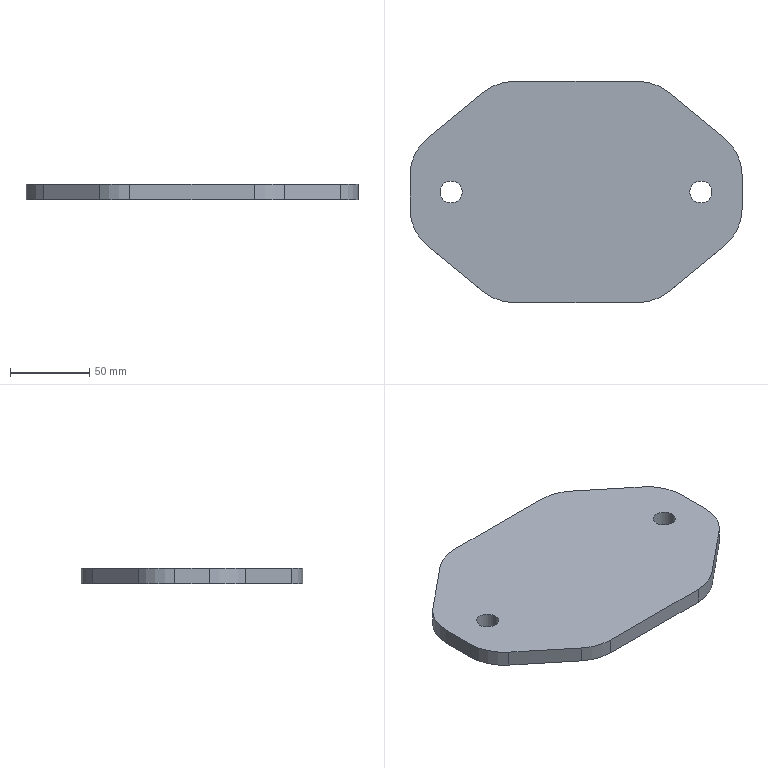Part | STEP file | VD-SYL0380DJ1006_1_1_2-3_VD-SYL | 1 solid | 22 faces | box 210 x 140 x 10 mm | volume 239785 mm3 | cylinder 12 | plane 10 | commonest cylinder face diameters 60 x8 14 x4
STEP:
#1=CARTESIAN_POINT('',(86.,0.,0.));
#2=VERTEX_POINT('',#1);
#3=CARTESIAN_POINT('',(72.,0.,0.));
#4=VERTEX_POINT('',#3);
#5=CARTESIAN_POINT('',(79.,0.,0.));
#6=DIRECTION('',(0.,0.,1.));
#7=DIRECTION('',(1.,0.,0.));
#8=AXIS2_PLACEMENT_3D('',#5,#6,#7);
#9=CIRCLE('',#8,7.);
#10=EDGE_CURVE('',#2,#4,#9,.T.);
#11=ORIENTED_EDGE('',*,*,#10,.F.);
#12=CARTESIAN_POINT('',(86.,0.,10.));
#13=VERTEX_POINT('',#12);
#14=CARTESIAN_POINT('',(86.,0.,10.));
#15=DIRECTION('',(0.,0.,-1.));
#16=VECTOR('',#15,1000.);
#17=LINE('',#14,#16);
#18=EDGE_CURVE('',#13,#2,#17,.T.);
#19=ORIENTED_EDGE('',*,*,#18,.F.);
#20=CARTESIAN_POINT('',(72.,0.,10.));
#21=VERTEX_POINT('',#20);
#22=CARTESIAN_POINT('',(79.,0.,10.));
#23=DIRECTION('',(0.,0.,-1.));
#24=DIRECTION('',(-1.,0.,0.));
#25=AXIS2_PLACEMENT_3D('',#22,#23,#24);
#26=CIRCLE('',#25,7.);
#27=EDGE_CURVE('',#21,#13,#26,.T.);
#28=ORIENTED_EDGE('',*,*,#27,.F.);
#29=CARTESIAN_POINT('',(72.,0.,10.));
#30=DIRECTION('',(0.,0.,-1.));
#31=VECTOR('',#30,1000.);
#32=LINE('',#29,#31);
#33=EDGE_CURVE('',#21,#4,#32,.T.);
#34=ORIENTED_EDGE('',*,*,#33,.T.);
#35=EDGE_LOOP('',(#11,#19,#28,#34));
#36=FACE_OUTER_BOUND('',#35,.T.);
#37=CARTESIAN_POINT('',(79.,0.,5.));
#38=DIRECTION('',(0.,0.,1.));
#39=DIRECTION('',(1.,0.,0.));
#40=AXIS2_PLACEMENT_3D('',#37,#38,#39);
#41=CYLINDRICAL_SURFACE('',#40,7.);
#42=ADVANCED_FACE('',(#36),#41,.F.);
#43=ORIENTED_EDGE('',*,*,#33,.F.);
#44=CARTESIAN_POINT('',(79.,0.,10.));
#45=DIRECTION('',(0.,0.,-1.));
#46=DIRECTION('',(1.,0.,0.));
#47=AXIS2_PLACEMENT_3D('',#44,#45,#46);
#48=CIRCLE('',#47,7.);
#49=EDGE_CURVE('',#13,#21,#48,.T.);
#50=ORIENTED_EDGE('',*,*,#49,.F.);
#51=ORIENTED_EDGE('',*,*,#18,.T.);
#52=CARTESIAN_POINT('',(79.,0.,0.));
#53=DIRECTION('',(0.,0.,1.));
#54=DIRECTION('',(-1.,0.,0.));
#55=AXIS2_PLACEMENT_3D('',#52,#53,#54);
#56=CIRCLE('',#55,7.);
#57=EDGE_CURVE('',#4,#2,#56,.T.);
#58=ORIENTED_EDGE('',*,*,#57,.F.);
#59=EDGE_LOOP('',(#43,#50,#51,#58));
#60=FACE_OUTER_BOUND('',#59,.T.);
#61=CARTESIAN_POINT('',(79.,0.,5.));
#62=DIRECTION('',(0.,0.,1.));
#63=DIRECTION('',(1.,0.,0.));
#64=AXIS2_PLACEMENT_3D('',#61,#62,#63);
#65=CYLINDRICAL_SURFACE('',#64,7.);
#66=ADVANCED_FACE('',(#60),#65,.F.);
#67=CARTESIAN_POINT('',(-72.,0.,0.));
#68=VERTEX_POINT('',#67);
#69=CARTESIAN_POINT('',(-86.,0.,0.));
#70=VERTEX_POINT('',#69);
#71=CARTESIAN_POINT('',(-79.,0.,0.));
#72=DIRECTION('',(0.,0.,1.));
#73=DIRECTION('',(1.,0.,0.));
#74=AXIS2_PLACEMENT_3D('',#71,#72,#73);
#75=CIRCLE('',#74,7.);
#76=EDGE_CURVE('',#68,#70,#75,.T.);
#77=ORIENTED_EDGE('',*,*,#76,.F.);
#78=CARTESIAN_POINT('',(-72.,0.,10.));
#79=VERTEX_POINT('',#78);
#80=CARTESIAN_POINT('',(-72.,0.,10.));
#81=DIRECTION('',(0.,0.,-1.));
#82=VECTOR('',#81,1000.);
#83=LINE('',#80,#82);
#84=EDGE_CURVE('',#79,#68,#83,.T.);
#85=ORIENTED_EDGE('',*,*,#84,.F.);
#86=CARTESIAN_POINT('',(-86.,0.,10.));
#87=VERTEX_POINT('',#86);
#88=CARTESIAN_POINT('',(-79.,0.,10.));
#89=DIRECTION('',(0.,0.,-1.));
#90=DIRECTION('',(-1.,0.,0.));
#91=AXIS2_PLACEMENT_3D('',#88,#89,#90);
#92=CIRCLE('',#91,7.);
#93=EDGE_CURVE('',#87,#79,#92,.T.);
#94=ORIENTED_EDGE('',*,*,#93,.F.);
#95=CARTESIAN_POINT('',(-86.,0.,10.));
#96=DIRECTION('',(0.,0.,-1.));
#97=VECTOR('',#96,1000.);
#98=LINE('',#95,#97);
#99=EDGE_CURVE('',#87,#70,#98,.T.);
#100=ORIENTED_EDGE('',*,*,#99,.T.);
#101=EDGE_LOOP('',(#77,#85,#94,#100));
#102=FACE_OUTER_BOUND('',#101,.T.);
#103=CARTESIAN_POINT('',(-79.,0.,5.));
#104=DIRECTION('',(0.,0.,1.));
#105=DIRECTION('',(1.,0.,0.));
#106=AXIS2_PLACEMENT_3D('',#103,#104,#105);
#107=CYLINDRICAL_SURFACE('',#106,7.);
#108=ADVANCED_FACE('',(#102),#107,.F.);
#109=ORIENTED_EDGE('',*,*,#99,.F.);
#110=CARTESIAN_POINT('',(-79.,0.,10.));
#111=DIRECTION('',(0.,0.,-1.));
#112=DIRECTION('',(1.,0.,0.));
#113=AXIS2_PLACEMENT_3D('',#110,#111,#112);
#114=CIRCLE('',#113,7.);
#115=EDGE_CURVE('',#79,#87,#114,.T.);
#116=ORIENTED_EDGE('',*,*,#115,.F.);
#117=ORIENTED_EDGE('',*,*,#84,.T.);
#118=CARTESIAN_POINT('',(-79.,0.,0.));
#119=DIRECTION('',(0.,0.,1.));
#120=DIRECTION('',(-1.,0.,0.));
#121=AXIS2_PLACEMENT_3D('',#118,#119,#120);
#122=CIRCLE('',#121,7.);
#123=EDGE_CURVE('',#70,#68,#122,.T.);
#124=ORIENTED_EDGE('',*,*,#123,.F.);
#125=EDGE_LOOP('',(#109,#116,#117,#124));
#126=FACE_OUTER_BOUND('',#125,.T.);
#127=CARTESIAN_POINT('',(-79.,0.,5.));
#128=DIRECTION('',(0.,0.,1.));
#129=DIRECTION('',(1.,0.,0.));
#130=AXIS2_PLACEMENT_3D('',#127,#128,#129);
#131=CYLINDRICAL_SURFACE('',#130,7.);
#132=ADVANCED_FACE('',(#126),#131,.F.);
#133=CARTESIAN_POINT('',(105.,-10.784,0.));
#134=VERTEX_POINT('',#133);
#135=CARTESIAN_POINT('',(93.997,-34.002,0.));
#136=VERTEX_POINT('',#135);
#137=CARTESIAN_POINT('',(75.,-10.784,0.));
#138=DIRECTION('',(0.,0.,-1.));
#139=DIRECTION('',(1.,0.,0.));
#140=AXIS2_PLACEMENT_3D('',#137,#138,#139);
#141=CIRCLE('',#140,30.);
#142=EDGE_CURVE('',#134,#136,#141,.T.);
#143=ORIENTED_EDGE('',*,*,#142,.F.);
#144=CARTESIAN_POINT('',(105.,-10.784,10.));
#145=VERTEX_POINT('',#144);
#146=CARTESIAN_POINT('',(105.,-10.784,0.));
#147=DIRECTION('',(0.,0.,1.));
#148=VECTOR('',#147,1000.);
#149=LINE('',#146,#148);
#150=EDGE_CURVE('',#134,#145,#149,.T.);
#151=ORIENTED_EDGE('',*,*,#150,.T.);
#152=CARTESIAN_POINT('',(93.997,-34.002,10.));
#153=VERTEX_POINT('',#152);
#154=CARTESIAN_POINT('',(75.,-10.784,10.));
#155=DIRECTION('',(0.,0.,1.));
#156=DIRECTION('',(0.6332,-0.774,0.));
#157=AXIS2_PLACEMENT_3D('',#154,#155,#156);
#158=CIRCLE('',#157,30.);
#159=EDGE_CURVE('',#153,#145,#158,.T.);
#160=ORIENTED_EDGE('',*,*,#159,.F.);
#161=CARTESIAN_POINT('',(93.997,-34.002,10.));
#162=DIRECTION('',(0.,0.,-1.));
#163=VECTOR('',#162,1000.);
#164=LINE('',#161,#163);
#165=EDGE_CURVE('',#153,#136,#164,.T.);
#166=ORIENTED_EDGE('',*,*,#165,.T.);
#167=EDGE_LOOP('',(#143,#151,#160,#166));
#168=FACE_OUTER_BOUND('',#167,.T.);
#169=CARTESIAN_POINT('',(75.,-10.784,47.084));
#170=DIRECTION('',(0.,0.,-1.));
#171=DIRECTION('',(-1.,0.,0.));
#172=AXIS2_PLACEMENT_3D('',#169,#170,#171);
#173=CYLINDRICAL_SURFACE('',#172,30.);
#174=ADVANCED_FACE('',(#168),#173,.T.);
#175=CARTESIAN_POINT('',(58.288,-63.219,10.));
#176=VERTEX_POINT('',#175);
#177=CARTESIAN_POINT('',(58.288,-63.219,10.));
#178=DIRECTION('',(0.774,0.6332,0.));
#179=VECTOR('',#178,1000.);
#180=LINE('',#177,#179);
#181=EDGE_CURVE('',#176,#153,#180,.T.);
#182=ORIENTED_EDGE('',*,*,#181,.F.);
#183=CARTESIAN_POINT('',(58.288,-63.219,0.));
#184=VERTEX_POINT('',#183);
#185=CARTESIAN_POINT('',(58.288,-63.219,0.));
#186=DIRECTION('',(0.,0.,1.));
#187=VECTOR('',#186,1000.);
#188=LINE('',#185,#187);
#189=EDGE_CURVE('',#184,#176,#188,.T.);
#190=ORIENTED_EDGE('',*,*,#189,.F.);
#191=CARTESIAN_POINT('',(93.997,-34.002,0.));
#192=DIRECTION('',(-0.774,-0.6332,0.));
#193=VECTOR('',#192,1000.);
#194=LINE('',#191,#193);
#195=EDGE_CURVE('',#136,#184,#194,.T.);
#196=ORIENTED_EDGE('',*,*,#195,.F.);
#197=ORIENTED_EDGE('',*,*,#165,.F.);
#198=EDGE_LOOP('',(#182,#190,#196,#197));
#199=FACE_OUTER_BOUND('',#198,.T.);
#200=CARTESIAN_POINT('',(77.5,-47.5,5.));
#201=DIRECTION('',(-0.6332,0.774,0.));
#202=DIRECTION('',(0.,0.,1.));
#203=AXIS2_PLACEMENT_3D('',#200,#201,#202);
#204=PLANE('',#203);
#205=ADVANCED_FACE('',(#199),#204,.F.);
#206=CARTESIAN_POINT('',(39.291,-70.,0.));
#207=VERTEX_POINT('',#206);
#208=CARTESIAN_POINT('',(39.291,-40.,0.));
#209=DIRECTION('',(0.,0.,-1.));
#210=DIRECTION('',(0.6332,-0.774,0.));
#211=AXIS2_PLACEMENT_3D('',#208,#209,#210);
#212=CIRCLE('',#211,30.);
#213=EDGE_CURVE('',#184,#207,#212,.T.);
#214=ORIENTED_EDGE('',*,*,#213,.F.);
#215=ORIENTED_EDGE('',*,*,#189,.T.);
#216=CARTESIAN_POINT('',(39.291,-70.,10.));
#217=VERTEX_POINT('',#216);
#218=CARTESIAN_POINT('',(39.291,-40.,10.));
#219=DIRECTION('',(0.,0.,1.));
#220=DIRECTION('',(0.,-1.,0.));
#221=AXIS2_PLACEMENT_3D('',#218,#219,#220);
#222=CIRCLE('',#221,30.);
#223=EDGE_CURVE('',#217,#176,#222,.T.);
#224=ORIENTED_EDGE('',*,*,#223,.F.);
#225=CARTESIAN_POINT('',(39.291,-70.,10.));
#226=DIRECTION('',(0.,0.,-1.));
#227=VECTOR('',#226,1000.);
#228=LINE('',#225,#227);
#229=EDGE_CURVE('',#217,#207,#228,.T.);
#230=ORIENTED_EDGE('',*,*,#229,.T.);
#231=EDGE_LOOP('',(#214,#215,#224,#230));
#232=FACE_OUTER_BOUND('',#231,.T.);
#233=CARTESIAN_POINT('',(39.291,-40.,47.084));
#234=DIRECTION('',(0.,0.,-1.));
#235=DIRECTION('',(-1.,0.,0.));
#236=AXIS2_PLACEMENT_3D('',#233,#234,#235);
#237=CYLINDRICAL_SURFACE('',#236,30.);
#238=ADVANCED_FACE('',(#232),#237,.T.);
#239=CARTESIAN_POINT('',(-39.291,-70.,10.));
#240=VERTEX_POINT('',#239);
#241=CARTESIAN_POINT('',(39.291,-70.,10.));
#242=DIRECTION('',(-1.,0.,0.));
#243=VECTOR('',#242,1000.);
#244=LINE('',#241,#243);
#245=EDGE_CURVE('',#217,#240,#244,.T.);
#246=ORIENTED_EDGE('',*,*,#245,.T.);
#247=CARTESIAN_POINT('',(-39.291,-70.,0.));
#248=VERTEX_POINT('',#247);
#249=CARTESIAN_POINT('',(-39.291,-70.,0.));
#250=DIRECTION('',(0.,0.,1.));
#251=VECTOR('',#250,1000.);
#252=LINE('',#249,#251);
#253=EDGE_CURVE('',#248,#240,#252,.T.);
#254=ORIENTED_EDGE('',*,*,#253,.F.);
#255=CARTESIAN_POINT('',(-39.291,-70.,0.));
#256=DIRECTION('',(1.,0.,0.));
#257=VECTOR('',#256,1000.);
#258=LINE('',#255,#257);
#259=EDGE_CURVE('',#248,#207,#258,.T.);
#260=ORIENTED_EDGE('',*,*,#259,.T.);
#261=ORIENTED_EDGE('',*,*,#229,.F.);
#262=EDGE_LOOP('',(#246,#254,#260,#261));
#263=FACE_OUTER_BOUND('',#262,.T.);
#264=CARTESIAN_POINT('',(0.,-70.,5.));
#265=DIRECTION('',(0.,1.,0.));
#266=DIRECTION('',(1.,0.,0.));
#267=AXIS2_PLACEMENT_3D('',#264,#265,#266);
#268=PLANE('',#267);
#269=ADVANCED_FACE('',(#263),#268,.F.);
#270=CARTESIAN_POINT('',(-58.288,-63.219,0.));
#271=VERTEX_POINT('',#270);
#272=CARTESIAN_POINT('',(-39.291,-40.,0.));
#273=DIRECTION('',(0.,0.,-1.));
#274=DIRECTION('',(0.,-1.,0.));
#275=AXIS2_PLACEMENT_3D('',#272,#273,#274);
#276=CIRCLE('',#275,30.);
#277=EDGE_CURVE('',#248,#271,#276,.T.);
#278=ORIENTED_EDGE('',*,*,#277,.F.);
#279=ORIENTED_EDGE('',*,*,#253,.T.);
#280=CARTESIAN_POINT('',(-58.288,-63.219,10.));
#281=VERTEX_POINT('',#280);
#282=CARTESIAN_POINT('',(-39.291,-40.,10.));
#283=DIRECTION('',(0.,0.,1.));
#284=DIRECTION('',(-0.6332,-0.774,0.));
#285=AXIS2_PLACEMENT_3D('',#282,#283,#284);
#286=CIRCLE('',#285,30.);
#287=EDGE_CURVE('',#281,#240,#286,.T.);
#288=ORIENTED_EDGE('',*,*,#287,.F.);
#289=CARTESIAN_POINT('',(-58.288,-63.219,10.));
#290=DIRECTION('',(0.,0.,-1.));
#291=VECTOR('',#290,1000.);
#292=LINE('',#289,#291);
#293=EDGE_CURVE('',#281,#271,#292,.T.);
#294=ORIENTED_EDGE('',*,*,#293,.T.);
#295=EDGE_LOOP('',(#278,#279,#288,#294));
#296=FACE_OUTER_BOUND('',#295,.T.);
#297=CARTESIAN_POINT('',(-39.291,-40.,47.084));
#298=DIRECTION('',(0.,0.,-1.));
#299=DIRECTION('',(-1.,0.,0.));
#300=AXIS2_PLACEMENT_3D('',#297,#298,#299);
#301=CYLINDRICAL_SURFACE('',#300,30.);
#302=ADVANCED_FACE('',(#296),#301,.T.);
#303=CARTESIAN_POINT('',(-93.997,-34.002,10.));
#304=VERTEX_POINT('',#303);
#305=CARTESIAN_POINT('',(-93.997,-34.002,10.));
#306=DIRECTION('',(0.774,-0.6332,0.));
#307=VECTOR('',#306,1000.);
#308=LINE('',#305,#307);
#309=EDGE_CURVE('',#304,#281,#308,.T.);
#310=ORIENTED_EDGE('',*,*,#309,.F.);
#311=CARTESIAN_POINT('',(-93.997,-34.002,0.));
#312=VERTEX_POINT('',#311);
#313=CARTESIAN_POINT('',(-93.997,-34.002,0.));
#314=DIRECTION('',(0.,0.,1.));
#315=VECTOR('',#314,1000.);
#316=LINE('',#313,#315);
#317=EDGE_CURVE('',#312,#304,#316,.T.);
#318=ORIENTED_EDGE('',*,*,#317,.F.);
#319=CARTESIAN_POINT('',(-58.288,-63.219,0.));
#320=DIRECTION('',(-0.774,0.6332,0.));
#321=VECTOR('',#320,1000.);
#322=LINE('',#319,#321);
#323=EDGE_CURVE('',#271,#312,#322,.T.);
#324=ORIENTED_EDGE('',*,*,#323,.F.);
#325=ORIENTED_EDGE('',*,*,#293,.F.);
#326=EDGE_LOOP('',(#310,#318,#324,#325));
#327=FACE_OUTER_BOUND('',#326,.T.);
#328=CARTESIAN_POINT('',(-77.5,-47.5,5.));
#329=DIRECTION('',(0.6332,0.774,0.));
#330=DIRECTION('',(0.,0.,-1.));
#331=AXIS2_PLACEMENT_3D('',#328,#329,#330);
#332=PLANE('',#331);
#333=ADVANCED_FACE('',(#327),#332,.F.);
#334=CARTESIAN_POINT('',(-105.,-10.784,0.));
#335=VERTEX_POINT('',#334);
#336=CARTESIAN_POINT('',(-75.,-10.784,0.));
#337=DIRECTION('',(0.,0.,-1.));
#338=DIRECTION('',(-0.6332,-0.774,0.));
#339=AXIS2_PLACEMENT_3D('',#336,#337,#338);
#340=CIRCLE('',#339,30.);
#341=EDGE_CURVE('',#312,#335,#340,.T.);
#342=ORIENTED_EDGE('',*,*,#341,.F.);
#343=ORIENTED_EDGE('',*,*,#317,.T.);
#344=CARTESIAN_POINT('',(-105.,-10.784,10.));
#345=VERTEX_POINT('',#344);
#346=CARTESIAN_POINT('',(-75.,-10.784,10.));
#347=DIRECTION('',(0.,0.,1.));
#348=DIRECTION('',(-1.,0.,0.));
#349=AXIS2_PLACEMENT_3D('',#346,#347,#348);
#350=CIRCLE('',#349,30.);
#351=EDGE_CURVE('',#345,#304,#350,.T.);
#352=ORIENTED_EDGE('',*,*,#351,.F.);
#353=CARTESIAN_POINT('',(-105.,-10.784,10.));
#354=DIRECTION('',(0.,0.,-1.));
#355=VECTOR('',#354,1000.);
#356=LINE('',#353,#355);
#357=EDGE_CURVE('',#345,#335,#356,.T.);
#358=ORIENTED_EDGE('',*,*,#357,.T.);
#359=EDGE_LOOP('',(#342,#343,#352,#358));
#360=FACE_OUTER_BOUND('',#359,.T.);
#361=CARTESIAN_POINT('',(-75.,-10.784,47.084));
#362=DIRECTION('',(0.,0.,-1.));
#363=DIRECTION('',(-1.,0.,0.));
#364=AXIS2_PLACEMENT_3D('',#361,#362,#363);
#365=CYLINDRICAL_SURFACE('',#364,30.);
#366=ADVANCED_FACE('',(#360),#365,.T.);
#367=CARTESIAN_POINT('',(-105.,10.784,0.));
#368=VERTEX_POINT('',#367);
#369=CARTESIAN_POINT('',(-105.,10.784,0.));
#370=DIRECTION('',(0.,-1.,0.));
#371=VECTOR('',#370,1000.);
#372=LINE('',#369,#371);
#373=EDGE_CURVE('',#368,#335,#372,.T.);
#374=ORIENTED_EDGE('',*,*,#373,.T.);
#375=ORIENTED_EDGE('',*,*,#357,.F.);
#376=CARTESIAN_POINT('',(-105.,10.784,10.));
#377=VERTEX_POINT('',#376);
#378=CARTESIAN_POINT('',(-105.,-10.784,10.));
#379=DIRECTION('',(0.,1.,0.));
#380=VECTOR('',#379,1000.);
#381=LINE('',#378,#380);
#382=EDGE_CURVE('',#345,#377,#381,.T.);
#383=ORIENTED_EDGE('',*,*,#382,.T.);
#384=CARTESIAN_POINT('',(-105.,10.784,0.));
#385=DIRECTION('',(0.,0.,1.));
#386=VECTOR('',#385,1000.);
#387=LINE('',#384,#386);
#388=EDGE_CURVE('',#368,#377,#387,.T.);
#389=ORIENTED_EDGE('',*,*,#388,.F.);
#390=EDGE_LOOP('',(#374,#375,#383,#389));
#391=FACE_OUTER_BOUND('',#390,.T.);
#392=CARTESIAN_POINT('',(-105.,0.,5.));
#393=DIRECTION('',(1.,0.,0.));
#394=DIRECTION('',(0.,1.,0.));
#395=AXIS2_PLACEMENT_3D('',#392,#393,#394);
#396=PLANE('',#395);
#397=ADVANCED_FACE('',(#391),#396,.F.);
#398=ORIENTED_EDGE('',*,*,#27,.T.);
#399=ORIENTED_EDGE('',*,*,#49,.T.);
#400=EDGE_LOOP('',(#398,#399));
#401=FACE_BOUND('',#400,.T.);
#402=ORIENTED_EDGE('',*,*,#93,.T.);
#403=ORIENTED_EDGE('',*,*,#115,.T.);
#404=EDGE_LOOP('',(#402,#403));
#405=FACE_BOUND('',#404,.T.);
#406=ORIENTED_EDGE('',*,*,#351,.T.);
#407=ORIENTED_EDGE('',*,*,#309,.T.);
#408=ORIENTED_EDGE('',*,*,#287,.T.);
#409=ORIENTED_EDGE('',*,*,#245,.F.);
#410=ORIENTED_EDGE('',*,*,#223,.T.);
#411=ORIENTED_EDGE('',*,*,#181,.T.);
#412=ORIENTED_EDGE('',*,*,#159,.T.);
#413=CARTESIAN_POINT('',(105.,10.784,10.));
#414=VERTEX_POINT('',#413);
#415=CARTESIAN_POINT('',(105.,10.784,10.));
#416=DIRECTION('',(0.,-1.,0.));
#417=VECTOR('',#416,1000.);
#418=LINE('',#415,#417);
#419=EDGE_CURVE('',#414,#145,#418,.T.);
#420=ORIENTED_EDGE('',*,*,#419,.F.);
#421=CARTESIAN_POINT('',(93.997,34.002,10.));
#422=VERTEX_POINT('',#421);
#423=CARTESIAN_POINT('',(75.,10.784,10.));
#424=DIRECTION('',(0.,0.,1.));
#425=DIRECTION('',(1.,0.,0.));
#426=AXIS2_PLACEMENT_3D('',#423,#424,#425);
#427=CIRCLE('',#426,30.);
#428=EDGE_CURVE('',#414,#422,#427,.T.);
#429=ORIENTED_EDGE('',*,*,#428,.T.);
#430=CARTESIAN_POINT('',(58.288,63.219,10.));
#431=VERTEX_POINT('',#430);
#432=CARTESIAN_POINT('',(93.997,34.002,10.));
#433=DIRECTION('',(-0.774,0.6332,0.));
#434=VECTOR('',#433,1000.);
#435=LINE('',#432,#434);
#436=EDGE_CURVE('',#422,#431,#435,.T.);
#437=ORIENTED_EDGE('',*,*,#436,.T.);
#438=CARTESIAN_POINT('',(39.291,70.,10.));
#439=VERTEX_POINT('',#438);
#440=CARTESIAN_POINT('',(39.291,40.,10.));
#441=DIRECTION('',(0.,0.,1.));
#442=DIRECTION('',(0.6332,0.774,0.));
#443=AXIS2_PLACEMENT_3D('',#440,#441,#442);
#444=CIRCLE('',#443,30.);
#445=EDGE_CURVE('',#431,#439,#444,.T.);
#446=ORIENTED_EDGE('',*,*,#445,.T.);
#447=CARTESIAN_POINT('',(-39.291,70.,10.));
#448=VERTEX_POINT('',#447);
#449=CARTESIAN_POINT('',(-39.291,70.,10.));
#450=DIRECTION('',(1.,0.,0.));
#451=VECTOR('',#450,1000.);
#452=LINE('',#449,#451);
#453=EDGE_CURVE('',#448,#439,#452,.T.);
#454=ORIENTED_EDGE('',*,*,#453,.F.);
#455=CARTESIAN_POINT('',(-58.288,63.219,10.));
#456=VERTEX_POINT('',#455);
#457=CARTESIAN_POINT('',(-39.291,40.,10.));
#458=DIRECTION('',(0.,0.,1.));
#459=DIRECTION('',(0.,1.,0.));
#460=AXIS2_PLACEMENT_3D('',#457,#458,#459);
#461=CIRCLE('',#460,30.);
#462=EDGE_CURVE('',#448,#456,#461,.T.);
#463=ORIENTED_EDGE('',*,*,#462,.T.);
#464=CARTESIAN_POINT('',(-93.997,34.002,10.));
#465=VERTEX_POINT('',#464);
#466=CARTESIAN_POINT('',(-58.288,63.219,10.));
#467=DIRECTION('',(-0.774,-0.6332,0.));
#468=VECTOR('',#467,1000.);
#469=LINE('',#466,#468);
#470=EDGE_CURVE('',#456,#465,#469,.T.);
#471=ORIENTED_EDGE('',*,*,#470,.T.);
#472=CARTESIAN_POINT('',(-75.,10.784,10.));
#473=DIRECTION('',(0.,0.,1.));
#474=DIRECTION('',(-0.6332,0.774,0.));
#475=AXIS2_PLACEMENT_3D('',#472,#473,#474);
#476=CIRCLE('',#475,30.);
#477=EDGE_CURVE('',#465,#377,#476,.T.);
#478=ORIENTED_EDGE('',*,*,#477,.T.);
#479=ORIENTED_EDGE('',*,*,#382,.F.);
#480=EDGE_LOOP('',(#406,#407,#408,#409,#410,#411,#412,#420,#429,#437,#446,#454,#463,#471,#478,#479));
#481=FACE_OUTER_BOUND('',#480,.T.);
#482=CARTESIAN_POINT('',(0.,0.,10.));
#483=DIRECTION('',(0.,0.,1.));
#484=DIRECTION('',(1.,0.,0.));
#485=AXIS2_PLACEMENT_3D('',#482,#483,#484);
#486=PLANE('',#485);
#487=ADVANCED_FACE('',(#401,#405,#481),#486,.T.);
#488=CARTESIAN_POINT('',(-58.288,63.219,0.));
#489=VERTEX_POINT('',#488);
#490=CARTESIAN_POINT('',(-39.291,70.,0.));
#491=VERTEX_POINT('',#490);
#492=CARTESIAN_POINT('',(-39.291,40.,0.));
#493=DIRECTION('',(0.,0.,-1.));
#494=DIRECTION('',(-0.6332,0.774,0.));
#495=AXIS2_PLACEMENT_3D('',#492,#493,#494);
#496=CIRCLE('',#495,30.);
#497=EDGE_CURVE('',#489,#491,#496,.T.);
#498=ORIENTED_EDGE('',*,*,#497,.F.);
#499=CARTESIAN_POINT('',(-58.288,63.219,0.));
#500=DIRECTION('',(0.,0.,1.));
#501=VECTOR('',#500,1000.);
#502=LINE('',#499,#501);
#503=EDGE_CURVE('',#489,#456,#502,.T.);
#504=ORIENTED_EDGE('',*,*,#503,.T.);
#505=ORIENTED_EDGE('',*,*,#462,.F.);
#506=CARTESIAN_POINT('',(-39.291,70.,10.));
#507=DIRECTION('',(0.,0.,-1.));
#508=VECTOR('',#507,1000.);
#509=LINE('',#506,#508);
#510=EDGE_CURVE('',#448,#491,#509,.T.);
#511=ORIENTED_EDGE('',*,*,#510,.T.);
#512=EDGE_LOOP('',(#498,#504,#505,#511));
#513=FACE_OUTER_BOUND('',#512,.T.);
#514=CARTESIAN_POINT('',(-39.291,40.,47.084));
#515=DIRECTION('',(0.,0.,-1.));
#516=DIRECTION('',(-1.,0.,0.));
#517=AXIS2_PLACEMENT_3D('',#514,#515,#516);
#518=CYLINDRICAL_SURFACE('',#517,30.);
#519=ADVANCED_FACE('',(#513),#518,.T.);
#520=CARTESIAN_POINT('',(-93.997,34.002,0.));
#521=VERTEX_POINT('',#520);
#522=CARTESIAN_POINT('',(-93.997,34.002,0.));
#523=DIRECTION('',(0.774,0.6332,0.));
#524=VECTOR('',#523,1000.);
#525=LINE('',#522,#524);
#526=EDGE_CURVE('',#521,#489,#525,.T.);
#527=ORIENTED_EDGE('',*,*,#526,.F.);
#528=CARTESIAN_POINT('',(-93.997,34.002,10.));
#529=DIRECTION('',(0.,0.,-1.));
#530=VECTOR('',#529,1000.);
#531=LINE('',#528,#530);
#532=EDGE_CURVE('',#465,#521,#531,.T.);
#533=ORIENTED_EDGE('',*,*,#532,.F.);
#534=ORIENTED_EDGE('',*,*,#470,.F.);
#535=ORIENTED_EDGE('',*,*,#503,.F.);
#536=EDGE_LOOP('',(#527,#533,#534,#535));
#537=FACE_OUTER_BOUND('',#536,.T.);
#538=CARTESIAN_POINT('',(-77.5,47.5,5.));
#539=DIRECTION('',(0.6332,-0.774,0.));
#540=DIRECTION('',(0.,0.,-1.));
#541=AXIS2_PLACEMENT_3D('',#538,#539,#540);
#542=PLANE('',#541);
#543=ADVANCED_FACE('',(#537),#542,.F.);
#544=CARTESIAN_POINT('',(-75.,10.784,0.));
#545=DIRECTION('',(0.,0.,-1.));
#546=DIRECTION('',(-1.,0.,0.));
#547=AXIS2_PLACEMENT_3D('',#544,#545,#546);
#548=CIRCLE('',#547,30.);
#549=EDGE_CURVE('',#368,#521,#548,.T.);
#550=ORIENTED_EDGE('',*,*,#549,.F.);
#551=ORIENTED_EDGE('',*,*,#388,.T.);
#552=ORIENTED_EDGE('',*,*,#477,.F.);
#553=ORIENTED_EDGE('',*,*,#532,.T.);
#554=EDGE_LOOP('',(#550,#551,#552,#553));
#555=FACE_OUTER_BOUND('',#554,.T.);
#556=CARTESIAN_POINT('',(-75.,10.784,47.084));
#557=DIRECTION('',(0.,0.,-1.));
#558=DIRECTION('',(-1.,0.,0.));
#559=AXIS2_PLACEMENT_3D('',#556,#557,#558);
#560=CYLINDRICAL_SURFACE('',#559,30.);
#561=ADVANCED_FACE('',(#555),#560,.T.);
#562=ORIENTED_EDGE('',*,*,#123,.T.);
#563=ORIENTED_EDGE('',*,*,#76,.T.);
#564=EDGE_LOOP('',(#562,#563));
#565=FACE_BOUND('',#564,.T.);
#566=ORIENTED_EDGE('',*,*,#57,.T.);
#567=ORIENTED_EDGE('',*,*,#10,.T.);
#568=EDGE_LOOP('',(#566,#567));
#569=FACE_BOUND('',#568,.T.);
#570=ORIENTED_EDGE('',*,*,#526,.T.);
#571=ORIENTED_EDGE('',*,*,#497,.T.);
#572=CARTESIAN_POINT('',(39.291,70.,0.));
#573=VERTEX_POINT('',#572);
#574=CARTESIAN_POINT('',(39.291,70.,0.));
#575=DIRECTION('',(-1.,0.,0.));
#576=VECTOR('',#575,1000.);
#577=LINE('',#574,#576);
#578=EDGE_CURVE('',#573,#491,#577,.T.);
#579=ORIENTED_EDGE('',*,*,#578,.F.);
#580=CARTESIAN_POINT('',(58.288,63.219,0.));
#581=VERTEX_POINT('',#580);
#582=CARTESIAN_POINT('',(39.291,40.,0.));
#583=DIRECTION('',(0.,0.,-1.));
#584=DIRECTION('',(0.,1.,0.));
#585=AXIS2_PLACEMENT_3D('',#582,#583,#584);
#586=CIRCLE('',#585,30.);
#587=EDGE_CURVE('',#573,#581,#586,.T.);
#588=ORIENTED_EDGE('',*,*,#587,.T.);
#589=CARTESIAN_POINT('',(93.997,34.002,0.));
#590=VERTEX_POINT('',#589);
#591=CARTESIAN_POINT('',(58.288,63.219,0.));
#592=DIRECTION('',(0.774,-0.6332,0.));
#593=VECTOR('',#592,1000.);
#594=LINE('',#591,#593);
#595=EDGE_CURVE('',#581,#590,#594,.T.);
#596=ORIENTED_EDGE('',*,*,#595,.T.);
#597=CARTESIAN_POINT('',(105.,10.784,0.));
#598=VERTEX_POINT('',#597);
#599=CARTESIAN_POINT('',(75.,10.784,0.));
#600=DIRECTION('',(0.,0.,-1.));
#601=DIRECTION('',(0.6332,0.774,0.));
#602=AXIS2_PLACEMENT_3D('',#599,#600,#601);
#603=CIRCLE('',#602,30.);
#604=EDGE_CURVE('',#590,#598,#603,.T.);
#605=ORIENTED_EDGE('',*,*,#604,.T.);
#606=CARTESIAN_POINT('',(105.,-10.784,0.));
#607=DIRECTION('',(0.,1.,0.));
#608=VECTOR('',#607,1000.);
#609=LINE('',#606,#608);
#610=EDGE_CURVE('',#134,#598,#609,.T.);
#611=ORIENTED_EDGE('',*,*,#610,.F.);
#612=ORIENTED_EDGE('',*,*,#142,.T.);
#613=ORIENTED_EDGE('',*,*,#195,.T.);
#614=ORIENTED_EDGE('',*,*,#213,.T.);
#615=ORIENTED_EDGE('',*,*,#259,.F.);
#616=ORIENTED_EDGE('',*,*,#277,.T.);
#617=ORIENTED_EDGE('',*,*,#323,.T.);
#618=ORIENTED_EDGE('',*,*,#341,.T.);
#619=ORIENTED_EDGE('',*,*,#373,.F.);
#620=ORIENTED_EDGE('',*,*,#549,.T.);
#621=EDGE_LOOP('',(#570,#571,#579,#588,#596,#605,#611,#612,#613,#614,#615,#616,#617,#618,#619,#620));
#622=FACE_OUTER_BOUND('',#621,.T.);
#623=CARTESIAN_POINT('',(0.,0.,0.));
#624=DIRECTION('',(0.,0.,1.));
#625=DIRECTION('',(1.,0.,0.));
#626=AXIS2_PLACEMENT_3D('',#623,#624,#625);
#627=PLANE('',#626);
#628=ADVANCED_FACE('',(#565,#569,#622),#627,.F.);
#629=ORIENTED_EDGE('',*,*,#419,.T.);
#630=ORIENTED_EDGE('',*,*,#150,.F.);
#631=ORIENTED_EDGE('',*,*,#610,.T.);
#632=CARTESIAN_POINT('',(105.,10.784,10.));
#633=DIRECTION('',(0.,0.,-1.));
#634=VECTOR('',#633,1000.);
#635=LINE('',#632,#634);
#636=EDGE_CURVE('',#414,#598,#635,.T.);
#637=ORIENTED_EDGE('',*,*,#636,.F.);
#638=EDGE_LOOP('',(#629,#630,#631,#637));
#639=FACE_OUTER_BOUND('',#638,.T.);
#640=CARTESIAN_POINT('',(105.,0.,5.));
#641=DIRECTION('',(-1.,0.,0.));
#642=DIRECTION('',(0.,0.,1.));
#643=AXIS2_PLACEMENT_3D('',#640,#641,#642);
#644=PLANE('',#643);
#645=ADVANCED_FACE('',(#639),#644,.F.);
#646=ORIENTED_EDGE('',*,*,#604,.F.);
#647=CARTESIAN_POINT('',(93.997,34.002,0.));
#648=DIRECTION('',(0.,0.,1.));
#649=VECTOR('',#648,1000.);
#650=LINE('',#647,#649);
#651=EDGE_CURVE('',#590,#422,#650,.T.);
#652=ORIENTED_EDGE('',*,*,#651,.T.);
#653=ORIENTED_EDGE('',*,*,#428,.F.);
#654=ORIENTED_EDGE('',*,*,#636,.T.);
#655=EDGE_LOOP('',(#646,#652,#653,#654));
#656=FACE_OUTER_BOUND('',#655,.T.);
#657=CARTESIAN_POINT('',(75.,10.784,47.084));
#658=DIRECTION('',(0.,0.,-1.));
#659=DIRECTION('',(-1.,0.,0.));
#660=AXIS2_PLACEMENT_3D('',#657,#658,#659);
#661=CYLINDRICAL_SURFACE('',#660,30.);
#662=ADVANCED_FACE('',(#656),#661,.T.);
#663=ORIENTED_EDGE('',*,*,#595,.F.);
#664=CARTESIAN_POINT('',(58.288,63.219,10.));
#665=DIRECTION('',(0.,0.,-1.));
#666=VECTOR('',#665,1000.);
#667=LINE('',#664,#666);
#668=EDGE_CURVE('',#431,#581,#667,.T.);
#669=ORIENTED_EDGE('',*,*,#668,.F.);
#670=ORIENTED_EDGE('',*,*,#436,.F.);
#671=ORIENTED_EDGE('',*,*,#651,.F.);
#672=EDGE_LOOP('',(#663,#669,#670,#671));
#673=FACE_OUTER_BOUND('',#672,.T.);
#674=CARTESIAN_POINT('',(77.5,47.5,5.));
#675=DIRECTION('',(-0.6332,-0.774,0.));
#676=DIRECTION('',(-0.774,0.6332,0.));
#677=AXIS2_PLACEMENT_3D('',#674,#675,#676);
#678=PLANE('',#677);
#679=ADVANCED_FACE('',(#673),#678,.F.);
#680=ORIENTED_EDGE('',*,*,#587,.F.);
#681=CARTESIAN_POINT('',(39.291,70.,0.));
#682=DIRECTION('',(0.,0.,1.));
#683=VECTOR('',#682,1000.);
#684=LINE('',#681,#683);
#685=EDGE_CURVE('',#573,#439,#684,.T.);
#686=ORIENTED_EDGE('',*,*,#685,.T.);
#687=ORIENTED_EDGE('',*,*,#445,.F.);
#688=ORIENTED_EDGE('',*,*,#668,.T.);
#689=EDGE_LOOP('',(#680,#686,#687,#688));
#690=FACE_OUTER_BOUND('',#689,.T.);
#691=CARTESIAN_POINT('',(39.291,40.,47.084));
#692=DIRECTION('',(0.,0.,-1.));
#693=DIRECTION('',(-1.,0.,0.));
#694=AXIS2_PLACEMENT_3D('',#691,#692,#693);
#695=CYLINDRICAL_SURFACE('',#694,30.);
#696=ADVANCED_FACE('',(#690),#695,.T.);
#697=ORIENTED_EDGE('',*,*,#578,.T.);
#698=ORIENTED_EDGE('',*,*,#510,.F.);
#699=ORIENTED_EDGE('',*,*,#453,.T.);
#700=ORIENTED_EDGE('',*,*,#685,.F.);
#701=EDGE_LOOP('',(#697,#698,#699,#700));
#702=FACE_OUTER_BOUND('',#701,.T.);
#703=CARTESIAN_POINT('',(0.,70.,5.));
#704=DIRECTION('',(0.,-1.,0.));
#705=DIRECTION('',(0.,0.,-1.));
#706=AXIS2_PLACEMENT_3D('',#703,#704,#705);
#707=PLANE('',#706);
#708=ADVANCED_FACE('',(#702),#707,.F.);
#709=CLOSED_SHELL('',(#42,#66,#108,#132,#174,#205,#238,#269,#302,#333,#366,#397,#487,#519,#543,#561,#628,#645,#662,#679,#696,#708));
#710=MANIFOLD_SOLID_BREP('',#709);
#711=CARTESIAN_POINT('',(0.,0.,0.));
#712=DIRECTION('',(0.,0.,1.));
#713=DIRECTION('',(1.,0.,0.));
#714=AXIS2_PLACEMENT_3D('',#711,#712,#713);
#715=(LENGTH_UNIT()NAMED_UNIT(*)SI_UNIT(.MILLI.,.METRE.));
#716=UNCERTAINTY_MEASURE_WITH_UNIT(LENGTH_MEASURE(0.00001),#715,'','');
#717=(NAMED_UNIT(*)PLANE_ANGLE_UNIT()SI_UNIT($,.RADIAN.));
#718=(NAMED_UNIT(*)SI_UNIT($,.STERADIAN.)SOLID_ANGLE_UNIT());
#719=(GEOMETRIC_REPRESENTATION_CONTEXT(3)GLOBAL_UNCERTAINTY_ASSIGNED_CONTEXT((#716))GLOBAL_UNIT_ASSIGNED_CONTEXT((#715,#717,#718))REPRESENTATION_CONTEXT('',''));
#720=ADVANCED_BREP_SHAPE_REPRESENTATION('',(#710,#714),#719);